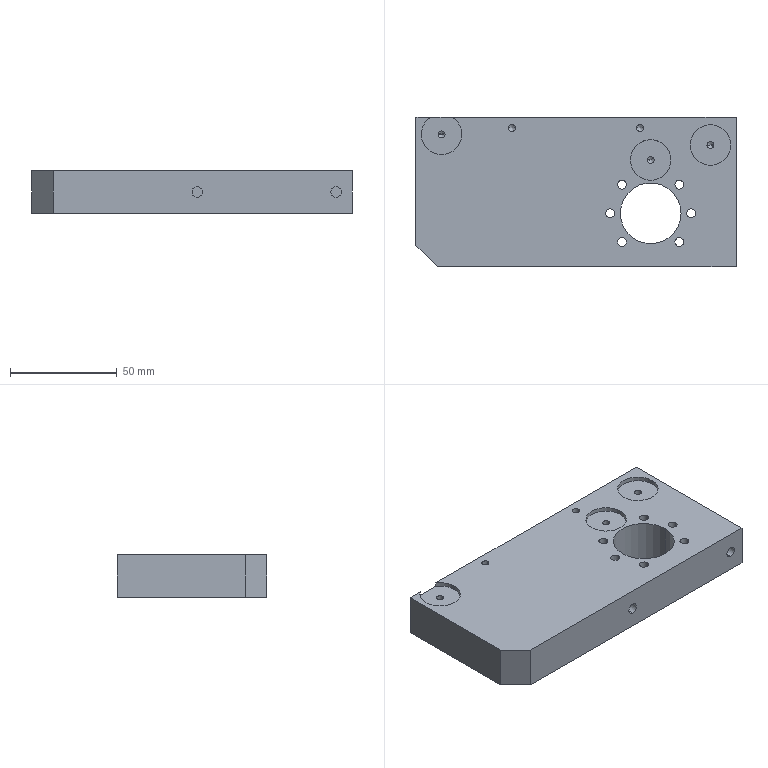Part | STEP file | Rear rail (left) | 1 solid | 78 faces | box 150 x 70 x 20 mm | volume 191088 mm3 | cylinder 47 | cone 16 | plane 15 | commonest cylinder face diameters 4.2 x18 3.3 x10 19 x7 4 x6 5 x4 28.5 x2